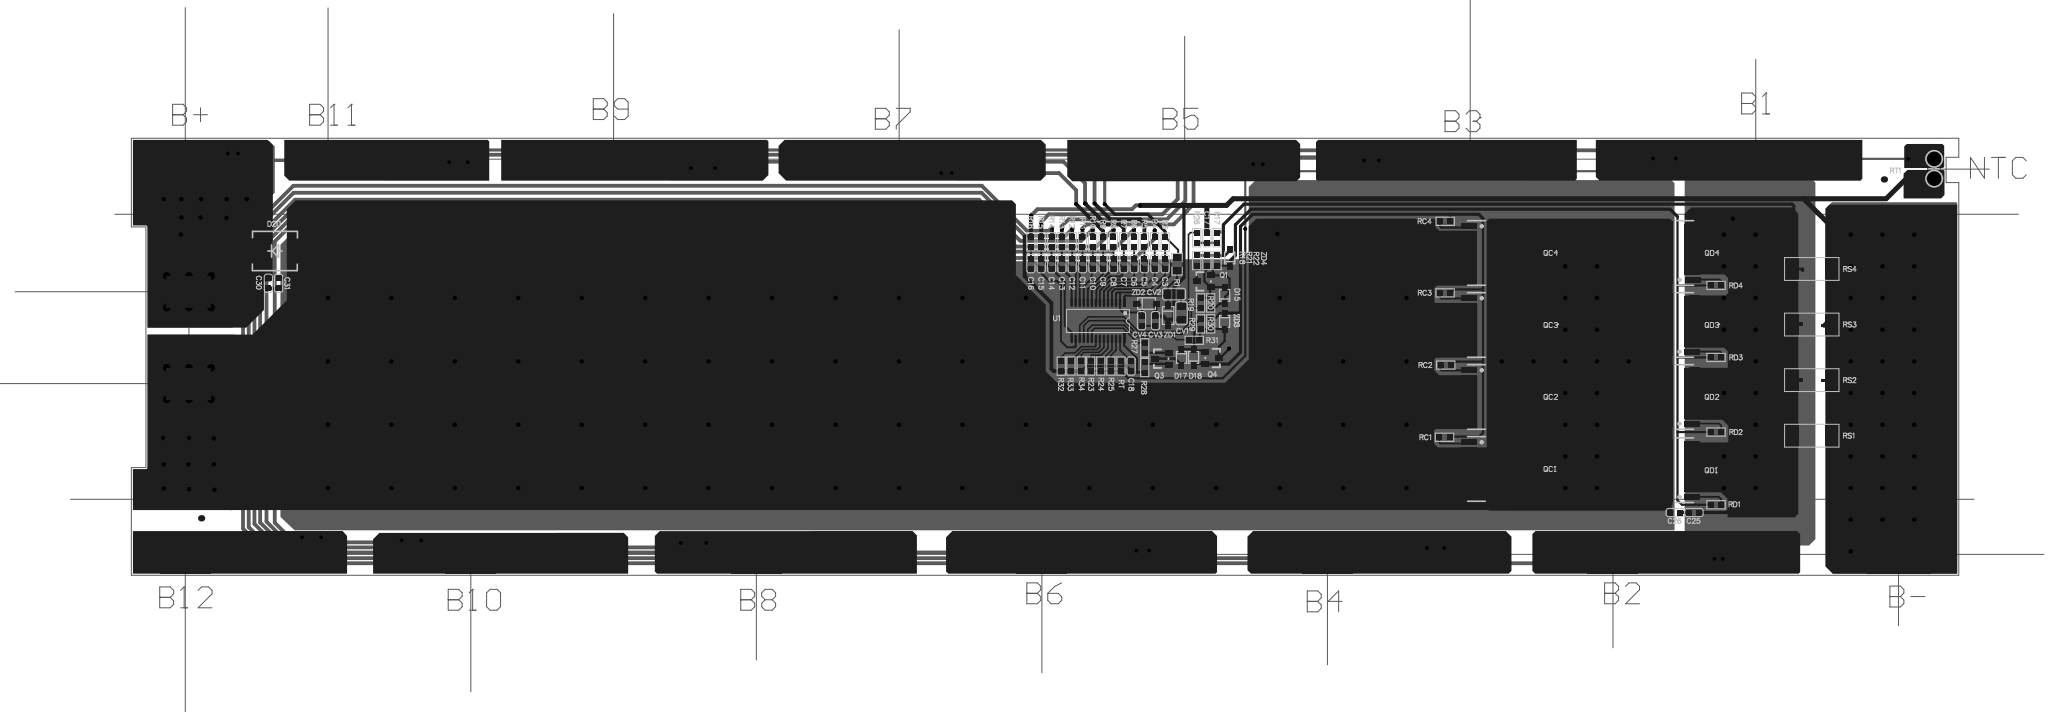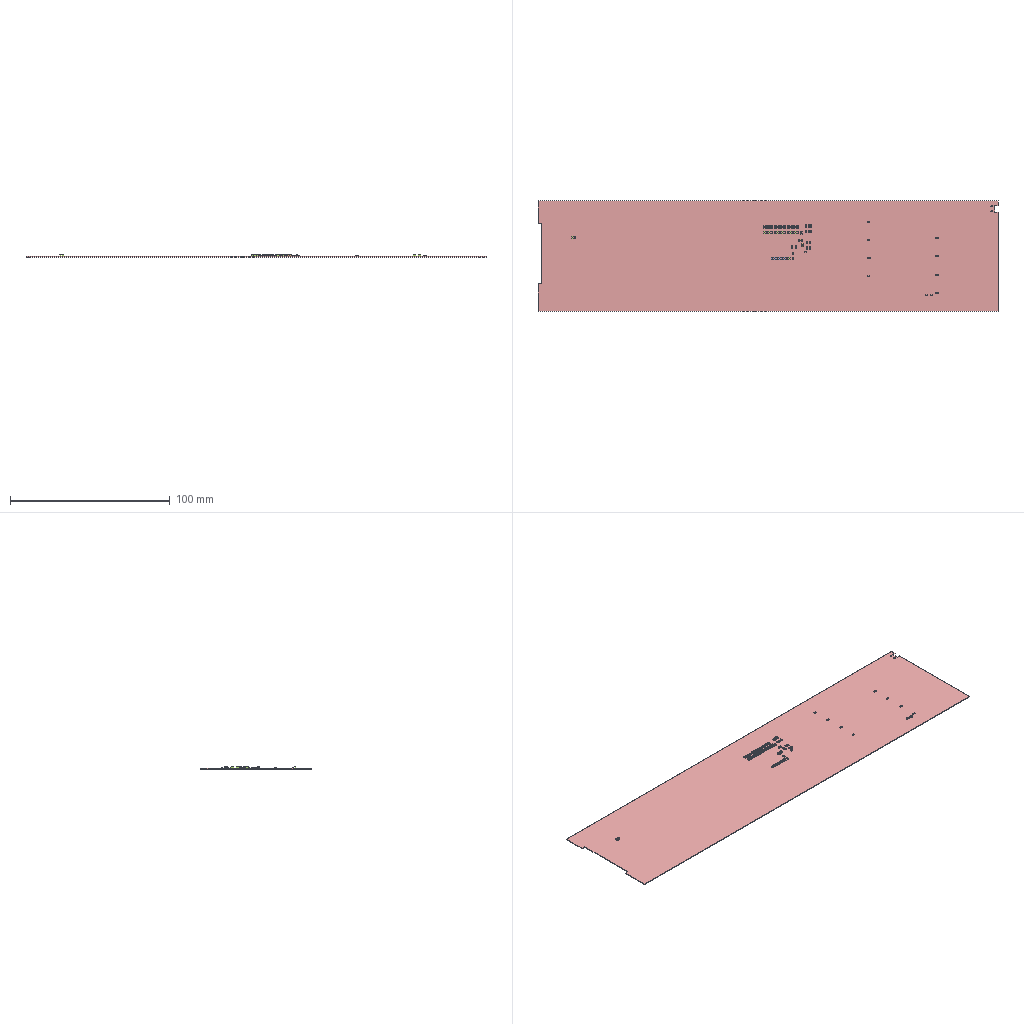Circuit board layout | Altium Designer | box 288 x 69 x 1.3 mm
Layer stack:
# Altium Designer layer stack of  (unit mm; dielectric type: 0 none, 1 core, 2 prepreg, 3 surface material)
index,name,kind,layer,copper_thickness_mm,dielectric_type,dielectric_thickness_mm,dielectric_material,dielectric_constant
0,Top Paste,other,,,,,,
1,Top Overlay,other,,,,,,
2,Top Solder,dielectric,,,3,0.0102,Solder Resist,3.5
3,Top Layer,copper,Top Layer,0.0356,,,,
4,Dielectric 1,dielectric,,,0,0.32,FR-4,4.8
5,Bottom Layer,copper,Bottom Layer,0.0356,,,,
6,Bottom Solder,dielectric,,,3,0.0102,Solder Resist,3.5
7,Bottom Overlay,other,,,,,,
8,Bottom Paste,other,,,,,,
# drill layer pairs: low layer,high layer
drill_pair,Top Layer,Bottom Layer
Part placement:
Designator,Comment,Layer,Footprint,Center-X(mm),Center-Y(mm),Rotation
ZD4,15V,TopLayer,SOD323,173.1,15.6,270
D15,1N4148,TopLayer,SOD323,172.3,9.7,270
QD1,NMOS,TopLayer,TOLL_123,242.643,-17.912,90
QD4,NMOS,TopLayer,TOLL_123,242.672,16.388,90
QD3,NMOS,TopLayer,TOLL_123,242.643,5.021,90
QD2,NMOS,TopLayer,TOLL_123,242.643,-6.349,90
QC3,NMOS,TopLayer,TOLL_123,214.133,5.021,270
QC2,NMOS,TopLayer,TOLL_123,214.133,-6.349,270
QC1,NMOS,TopLayer,TOLL_123,214.133,-17.712,270
QC4,NMOS,TopLayer,TOLL_123,214.133,16.388,270
ZD3,15V,TopLayer,SOD323,172.3,5.6,90
RT1,103AT B=3435,TopLayer,WK,284.117,29.69,270
RC4,47R,TopLayer,RES0603,207.055,21.388,270
RC3,47R,TopLayer,RES0603,207.045,10.088,270
RC2,47R,TopLayer,RES0603,207.145,-1.312,270
RC1,47R,TopLayer,RES0603,206.955,-12.712,270
R32,200K,TopLayer,RES0603,146.55,-1.482,0
ZD2,68V,TopLayer,SOD123,160,8.4,180
C15,104,TopLayer,CAP0603,143.395,14.7,0
C31,0.1uF,TopLayer,CAP0603,23.2,11.6,0
C30,0.1uF,TopLayer,CAP0603,21.6,11.6,180
RS4,,TopLayer,2512,264.845,13.863,90
RS3,,TopLayer,2512,264.845,5.088,90
RD4,47R,TopLayer,RES0603,249.745,11.263,90
RT,NC,TopLayer,RES0603,155.959,-1.467,180
R34,499K,TopLayer,RES0603,149.7,-1.457,0
RD3,47R,TopLayer,RES0603,249.745,-0.1123,90
RD2,47R,TopLayer,RES0603,249.745,-11.887,90
RD1,47R,TopLayer,RES0603,249.745,-23.362,90
R33,200K,TopLayer,RES0603,148.075,-1.457,0
R18,510R,TopLayer,RES0603,167.9,15.19,180
ZD1,68V,TopLayer,SOD123,163.4,6.5,90
U1,CW1143,TopLayer,SSOP-28-0.635,152.322,5.7,270
RS2,,TopLayer,2512,264.845,-3.687,90
RS1,,TopLayer,2512,264.845,-12.462,90
R31,1M,TopLayer,RES0603,167.51,2.6,90
R30,5.1M,TopLayer,RES0603,170.1,5.2,0
R29,5.1M,TopLayer,RES0603,168.5,5.2,0
R28,3M,TopLayer,RES0603,159.7,-1.7,180
R27,10K,TopLayer,RES0603,159.7,1.41,180
R25,22K,TopLayer,RES0603,154.368,-1.467,0
R24,41.2K,TopLayer,RES0603,152.776,-1.467,0
R23,270K,TopLayer,RES0603,151.185,-1.467,0
R22,5.1M,TopLayer,RES0603,171.1,15.2,180
R21,5.1M,TopLayer,RES0603,169.5,15.2,180
R20,NC,TopLayer,RES0603,170.1,8.5,0
R19,1K,TopLayer,RES0603,168.5,8.5,180
R26,10K,TopLayer,RES0603,167.9,18.8,180
R17,1K,TopLayer,RES0603,171.1,18.8,180
R16,2K,TopLayer,RES0603,141.767,18.15,0
R15,2K,TopLayer,RES0603,143.393,18.15,0
R14,2K,TopLayer,RES0603,145.019,18.15,0
R13,2K,TopLayer,RES0603,146.645,18.15,0
R12,2K,TopLayer,RES0603,148.27,18.15,0
R11,2K,TopLayer,RES0603,149.896,18.15,0
R10,2K,TopLayer,RES0603,151.522,18.15,0
R9,2K,TopLayer,RES0603,153.148,18.15,0
R8,2K,TopLayer,RES0603,154.774,18.15,0
R7,2K,TopLayer,RES0603,156.399,18.15,0
R6,2K,TopLayer,RES0603,158.025,18.15,0
R5,2K,TopLayer,RES0603,159.651,18.15,0
R4,2K,TopLayer,RES0603,161.277,18.15,0
R3,2K,TopLayer,RES0603,162.922,18.1,0
R1,2K,TopLayer,RES0805,164.8,14.584,270
Q4,MMBT5401,TopLayer,SOT-23-3,170.3,-0.2,270
Q3,MMBT5401,TopLayer,SOT-23-3,162.4,-0.3,90
Q1,MMBT5401,TopLayer,SOT-23-3,169.1,11.9,90
D20,RS3M,TopLayer,SMC,22.625,16.7,180
D18,1N4148,TopLayer,SOD323,167.4,-0.1,270
D17,1N4148,TopLayer,SOD323,165.5,-0.1,90
CV4,0.1uF,TopLayer,CAP0603,159.2,5.7,180
CV3,0.1uF,TopLayer,CAP0603,161.4,5.7,0
CV2,2.2uF,TopLayer,CAP0805,164.3,9.9,180
CV1,2.2uF,TopLayer,CAP0805,165.5,6.9,90
C26,0.1uF,TopLayer,CAP0603,243.32,-24.587,270
C25,0.1uF,TopLayer,CAP0603,246.255,-24.587,270
C18,104,TopLayer,CAP0603,157.55,-1.467,0
C17,104,TopLayer,CAP0603,169.5,18.8,180
C16,0.47uF,TopLayer,CAP0603,141.767,14.7,0
C14,104,TopLayer,CAP0603,145.022,14.7,0
C13,104,TopLayer,CAP0603,146.649,14.7,0
C12,104,TopLayer,CAP0603,148.276,14.7,0
C11,104,TopLayer,CAP0603,149.904,14.7,0
C10,104,TopLayer,CAP0603,151.531,14.7,0
C9,104,TopLayer,CAP0603,153.158,14.7,0
C8,104,TopLayer,CAP0603,154.786,14.7,0
C7,104,TopLayer,CAP0603,156.413,14.7,0
C6,104,TopLayer,CAP0603,158.04,14.7,0
C5,104,TopLayer,CAP0603,159.668,14.7,0
C4,104,TopLayer,CAP0603,161.295,14.7,0
C3,104,TopLayer,CAP0603,162.922,14.7,0
Pad and via stacks:
# Altium Designer via and pad stacks of  (unit mm). Each distinct definition once, with the count of objects using it.
# via: kind,start_layer,end_layer,hole_mm,diameter_mm,mode(0 simple;1 top-mid-bottom;2 full stack),diameter_per_layer,count,example_net
# pad: kind,layer,hole_mm,hole_type(0 round;1 square;2 slot),plating,top_size,top_shape(1 round;2 rect;3 octagon;9 rounded rect),mid_size,bottom_size,mode,footprint,size_per_layer,count,example
pad,Top Layer,0,0,plated,1x0.8,2,1x0.8,1x0.8,0,SOD323,,10,ZD4.2
pad,Top Layer,0,0,plated,0.83x0.88,2,0.83x0.88,0.83x0.88,0,CAP0603,,44,C3.1
pad,Top Layer,0,0,plated,1.27x1.016,2,1.27x1.016,1.27x1.016,0,RES0805,,2,R1.1
pad,Top Layer,0,0,plated,0.83x0.88,2,0.83x0.88,0.83x0.88,0,RES0603,,82,R3.2
pad,Top Layer,0,0,plated,9.9x8,2,9.9x8,9.9x8,0,TOLL_123,,8,QC4.3
pad,Top Layer,0,0,plated,0.8x8,2,0.8x8,0.8x8,0,TOLL_123,,8,QC4.2
pad,Top Layer,0,0,plated,1.7x0.8,2,1.7x0.8,1.7x0.8,0,TOLL_123,,56,QC4.2
pad,Top Layer,0,0,plated,2.5x0.8,2,2.5x0.8,2.5x0.8,0,TOLL_123,,8,QC4.1
pad,Top Layer,0,0,plated,2x3.2,2,2x3.2,2x3.2,0,2512,,8,RS1.1
pad,Top Layer,0,0,plated,1.4x0.4,1,1.4x0.4,1.4x0.4,0,SSOP-28-0.635,,26,U1.27
pad,Top Layer,0,0,plated,1.4x0.4,2,1.4x0.4,1.4x0.4,0,SSOP-28-0.635,,2,U1.28
pad,Top Layer,0,0,plated,0.9144x1.2,2,0.9144x1.2,0.9144x1.2,0,SOT-23-3,,9,Q3.3
pad,Top Layer,0,0,plated,8x6,2,8x6,8x6,0,,,12,609
pad,Top Layer,0,0,plated,10x6,2,10x6,10x6,0,,,2,597
pad,Top Layer,0,0,plated,1.27x1.1,2,1.27x1.1,1.27x1.1,0,CAP0805,,2,CV2.1
pad,Top Layer,0,0,plated,1.27x1.016,2,1.27x1.016,1.27x1.016,0,CAP0805,,2,CV2.2
pad,Top Layer,0,0,plated,2.44x3.62,2,2.44x3.62,2.44x3.62,0,SMC,,2,D20.1
pad,Top Layer,0,0,plated,1x0.8,2,1x0.8,1x0.8,0,SOD123,,4,ZD2.1
pad,Top Layer,0,0,plated,1x1,1,1x1,1x1,0,,,2,650
pad,Top Layer,0,0,plated,7x5,2,7x5,7x5,0,,,2,598
pad,Keep-Out Layer,0.075,0,plated,0.075x0.075,1,0.075x0.075,0.075x0.075,0,,,2,1
pad,Multi-Layer,1,0,plated,2.2x2.2,1,2.2x2.2,2.2x2.2,0,WK,,2,RT1.2
via,Top Layer,Bottom Layer,0.5,0.7,0,,152,P-
via,Top Layer,Bottom Layer,0.8,1.2,0,,14,P-
via,Top Layer,Bottom Layer,0.4,0.6,0,,44,B12
Copper pours:
name,layer,net,type(0 solid;1 hatched;2 none)
B-_L01_P088,Top Layer,B-,0
NETR23_2_L01_P093,Top Layer,NetR23_2,0
B-_L01_P092,Top Layer,B-,0
NONET_L-01_P-001,Top Layer,P-,0
NONET_L-01_P-001,Top Layer,B6,0
NONET_L-01_P-001,Top Layer,B2,0
NONET_L-01_P-001,Top Layer,B4,0
NONET_L-01_P-001,Top Layer,B8,0
NONET_L-01_P-001,Top Layer,B12,0
B+_L01_P081,Top Layer,B+,0
NONET_L-01_P-001,Top Layer,B7,0
NONET_L-01_P-001,Top Layer,B3,0
NONET_L-01_P-001,Top Layer,B1,0
NONET_L-01_P-001,Top Layer,B9,0
NONET_L-01_P-001,Top Layer,B5,0
NONET_L-01_P-001,Top Layer,B11,0
NONET_L-01_P-001,Top Layer,B10,0
NONET_L-01_P-001,Top Layer,P-,0
NONET_L-01_P-001,Top Layer,NetC25_1,0
P-_L02_P095,Bottom Layer,P-,0
B+_L02_P094,Bottom Layer,B+,0
P-_L02_P091,Bottom Layer,P-,0
NONET_L-01_P-001,Bottom Layer,NetC25_1,0
B-_L02_P089,Bottom Layer,B-,0
Design rules, without the lines most boards share:
# Altium Designer design rules of  (exported by Altium Designer, unit mm)
# columns: name | kind | enabled | priority | scope1 | scope2 | descriptor | typed fields (field=value)
Schematic Supply Nets | 41 | enabled | 1 | InNet('B-') | All | Supply Net(s)(InNet('B-')) |
NetAntennae | 56 | enabled | 1 | All | All | Net Antennae (Tolerance=0mm) (All) |
SilkToSilkClearance | 55 | enabled | 1 | All | All | Silk to Silk (Clearance=0.254mm) (All),(All) |
SilkToSolderMaskClearance | 54 | enabled | 1 | IsPad | All | Silk To Solder Mask (Clearance=0.254mm) (IsPad),(All) |
MinimumSolderMaskSliver | 53 | enabled | 1 | All | All | Minimum Solder Mask Sliver (Gap=0.254mm) (All),(All) |
HoleToHoleClearance | 52 | enabled | 1 | All | All | Hole To Hole Clearance (Gap=0.254mm) (All),(All) | gap=0.254
DiffPairsRouting | 51 | enabled | 1 | All | All | Differential Pairs Uncoupled Length using the Gap Constraints (Min=0.254mm) (Max=0.254mm) (Prefered=0.254mm)  and Width Constraints (Min=0.381mm) (Max=0.381mm) (Prefered=0.381mm) (All) |
HoleSize | 42 | enabled | 1 | All | All | Hole Size Constraint (Min=0.025mm) (Max=2.54mm) (All) |
Height | 50 | enabled | 1 | All | All | Height Constraint (Min=0mm) (Max=25.4mm) (Prefered=12.7mm) (All) | min_height=0 max_height=25.4
ComponentClearance | 24 | enabled | 1 | All | All | Component Clearance Constraint ( Horizontal Gap = 0.2mm, Vertical Gap = 0.254mm ) (All),(All)  | gap=0.2
SolderMaskExpansion | 13 | enabled | 1 | All | All | Solder Mask Expansion (Expansion =0.102mm) (All) | expansion=0.1016
PasteMaskExpansion | 14 | enabled | 1 | All | All | Paste Mask Expansion (Expansion =0mm) (All) | expansion=0
RoutingVias | 11 | enabled | 1 | All | All | Routing Via (MinHoleWidth=0.4mm) (MaxHoleWidth=0.4mm) (PreferredHoleWidth=0.4mm) (MinWidth=0.6mm) (MaxWidth=0.6mm) (PreferedWidth=0.6mm) (All) | via_min_hole=0.4 via_max_hole=0.4 via_preferred_diameter=0.6 via_preferred_hole=0.4
RoutingCorners | 10 | enabled | 1 | All | All | Routing Corners (Style=45-Degree) (Min Setback=2.54mm) (Max Setback=2.54mm) (All) |
Width | 2 | enabled | 1 | All | All | Width Constraint (Min=0.2mm) (Max=1mm) (Preferred=0.25mm) (All) |
PolygonConnect | 20 | enabled | 1 | All | All | Polygon Connect Rule(Direct Connect )(Conductor Width=0.254mm) (Relief Angle=90 Angle) (Entries=4) (Air Gap Width=0.254mm) (All),(All) | connect_style(0=relief,1=direct,2=none)=1 relief_conductor_width=0.254 relief_entries=4
PlaneClearance | 12 | enabled | 1 | All | All | Power Plane Clearance (Clearance =0.508mm) (All) | clearance=0.508
PlaneConnect | 6 | enabled | 1 | All | All | Power Plane Connect Rule(Relief Connect )(Expansion=0.508mm) (Conductor Width=0.254mm) (Air Gap=0.254mm) (Entries=4) (All) | relief_conductor_width=0.254 relief_entries=4 relief_expansion=0.508
Clearance | 0 | enabled | 1 | All | All | Clearance Constraint (Gap=0.2mm) (All),(All) | gap=0.2